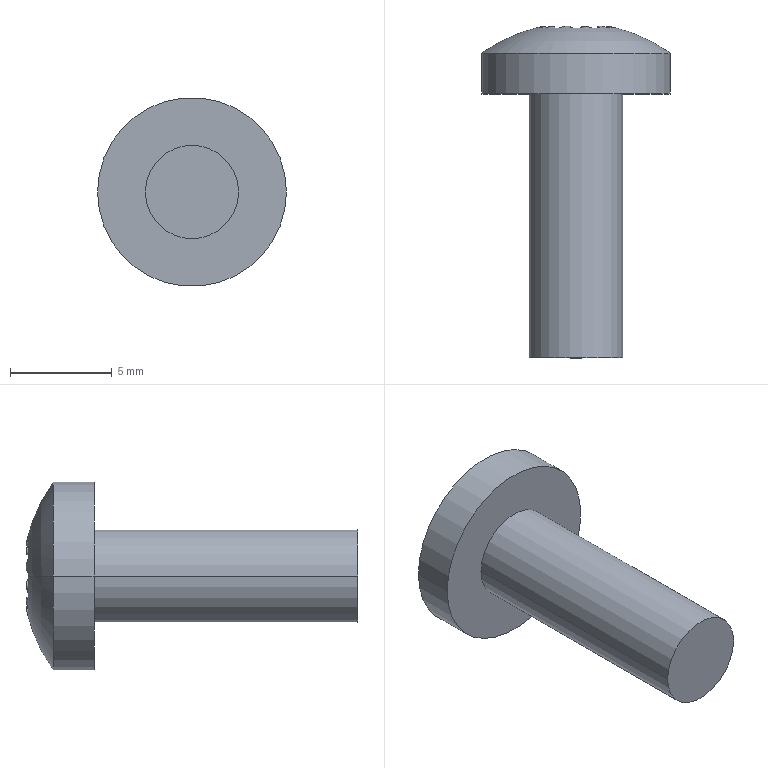Part | STEP file | 4_8X13Y | 1 solid | 33 faces | box 9.3 x 16.348 x 9.3 mm | volume 389.106 mm3 | cylinder 28 | plane 3 | sphere 2 | commonest cylinder face diameters 0.4 x18 4 x6 4.6 x2 9.3 x2